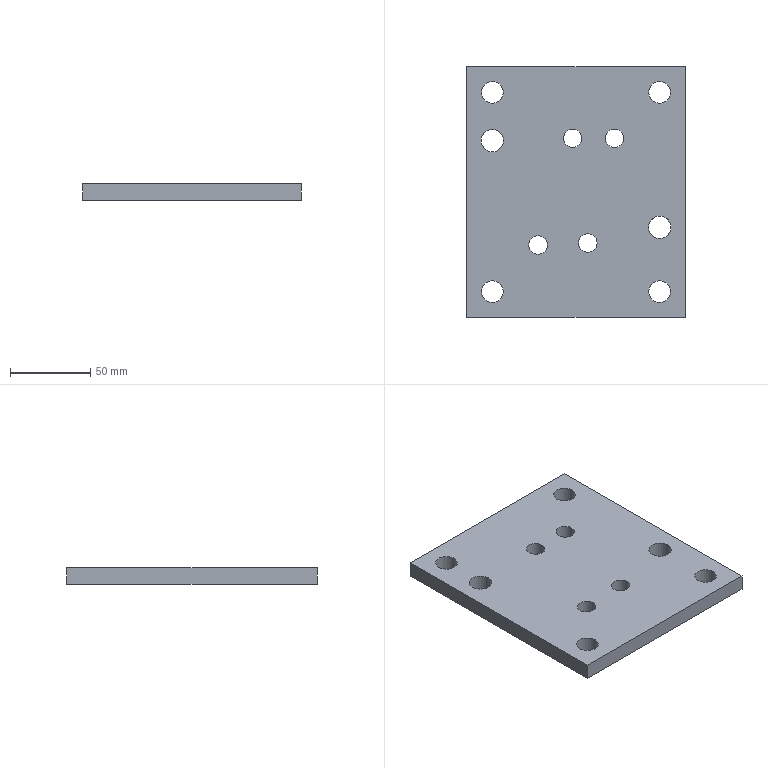Part | NX | features 6 2 | 1 solid | 16 faces | box 136 x 156 x 10 mm | volume 199200 mm3 | cylinder 10 | plane 6 | commonest cylinder face diameters 11.5 x4 13.5 x4 14.001 x2
STEP:
#1=CARTESIAN_POINT('',(3796.562,457.449,91.));
#2=VERTEX_POINT('',#1);
#3=CARTESIAN_POINT('',(3796.562,457.449,101.));
#4=VERTEX_POINT('',#3);
#5=CARTESIAN_POINT('',(3796.562,457.449,91.));
#6=DIRECTION('',(0.,0.,1.));
#7=VECTOR('',#6,1000.);
#8=LINE('',#5,#7);
#9=EDGE_CURVE('',#2,#4,#8,.T.);
#10=ORIENTED_EDGE('',*,*,#9,.F.);
#11=CARTESIAN_POINT('',(3660.562,457.449,91.));
#12=VERTEX_POINT('',#11);
#13=CARTESIAN_POINT('',(3728.562,457.449,91.));
#14=DIRECTION('',(1.,0.,0.));
#15=VECTOR('',#14,1000.);
#16=LINE('',#13,#15);
#17=EDGE_CURVE('',#12,#2,#16,.T.);
#18=ORIENTED_EDGE('',*,*,#17,.F.);
#19=CARTESIAN_POINT('',(3660.562,457.449,101.));
#20=VERTEX_POINT('',#19);
#21=CARTESIAN_POINT('',(3660.562,457.449,91.));
#22=DIRECTION('',(0.,0.,1.));
#23=VECTOR('',#22,1000.);
#24=LINE('',#21,#23);
#25=EDGE_CURVE('',#12,#20,#24,.T.);
#26=ORIENTED_EDGE('',*,*,#25,.T.);
#27=CARTESIAN_POINT('',(3728.562,457.449,101.));
#28=DIRECTION('',(-1.,0.,0.));
#29=VECTOR('',#28,1000.);
#30=LINE('',#27,#29);
#31=EDGE_CURVE('',#4,#20,#30,.T.);
#32=ORIENTED_EDGE('',*,*,#31,.F.);
#33=EDGE_LOOP('',(#10,#18,#26,#32));
#34=FACE_BOUND('',#33,.T.);
#35=CARTESIAN_POINT('',(3728.562,457.449,91.));
#36=DIRECTION('',(0.,1.,0.));
#37=DIRECTION('',(0.,0.,1.));
#38=AXIS2_PLACEMENT_3D('',#35,#36,#37);
#39=PLANE('',#38);
#40=ADVANCED_FACE('',(#34),#39,.T.);
#41=ORIENTED_EDGE('',*,*,#25,.F.);
#42=CARTESIAN_POINT('',(3660.562,301.449,91.));
#43=VERTEX_POINT('',#42);
#44=CARTESIAN_POINT('',(3660.562,379.449,91.));
#45=DIRECTION('',(0.,1.,0.));
#46=VECTOR('',#45,1000.);
#47=LINE('',#44,#46);
#48=EDGE_CURVE('',#43,#12,#47,.T.);
#49=ORIENTED_EDGE('',*,*,#48,.F.);
#50=CARTESIAN_POINT('',(3660.562,301.449,101.));
#51=VERTEX_POINT('',#50);
#52=CARTESIAN_POINT('',(3660.562,301.449,91.));
#53=DIRECTION('',(0.,0.,1.));
#54=VECTOR('',#53,1000.);
#55=LINE('',#52,#54);
#56=EDGE_CURVE('',#43,#51,#55,.T.);
#57=ORIENTED_EDGE('',*,*,#56,.T.);
#58=CARTESIAN_POINT('',(3660.562,379.449,101.));
#59=DIRECTION('',(0.,-1.,0.));
#60=VECTOR('',#59,1000.);
#61=LINE('',#58,#60);
#62=EDGE_CURVE('',#20,#51,#61,.T.);
#63=ORIENTED_EDGE('',*,*,#62,.F.);
#64=EDGE_LOOP('',(#41,#49,#57,#63));
#65=FACE_BOUND('',#64,.T.);
#66=CARTESIAN_POINT('',(3660.562,379.449,91.));
#67=DIRECTION('',(-1.,0.,0.));
#68=DIRECTION('',(0.,0.,-1.));
#69=AXIS2_PLACEMENT_3D('',#66,#67,#68);
#70=PLANE('',#69);
#71=ADVANCED_FACE('',(#65),#70,.T.);
#72=ORIENTED_EDGE('',*,*,#56,.F.);
#73=CARTESIAN_POINT('',(3796.562,301.449,91.));
#74=VERTEX_POINT('',#73);
#75=CARTESIAN_POINT('',(3728.562,301.449,91.));
#76=DIRECTION('',(-1.,0.,0.));
#77=VECTOR('',#76,1000.);
#78=LINE('',#75,#77);
#79=EDGE_CURVE('',#74,#43,#78,.T.);
#80=ORIENTED_EDGE('',*,*,#79,.F.);
#81=CARTESIAN_POINT('',(3796.562,301.449,101.));
#82=VERTEX_POINT('',#81);
#83=CARTESIAN_POINT('',(3796.562,301.449,91.));
#84=DIRECTION('',(0.,0.,1.));
#85=VECTOR('',#84,1000.);
#86=LINE('',#83,#85);
#87=EDGE_CURVE('',#74,#82,#86,.T.);
#88=ORIENTED_EDGE('',*,*,#87,.T.);
#89=CARTESIAN_POINT('',(3728.562,301.449,101.));
#90=DIRECTION('',(1.,0.,0.));
#91=VECTOR('',#90,1000.);
#92=LINE('',#89,#91);
#93=EDGE_CURVE('',#51,#82,#92,.T.);
#94=ORIENTED_EDGE('',*,*,#93,.F.);
#95=EDGE_LOOP('',(#72,#80,#88,#94));
#96=FACE_BOUND('',#95,.T.);
#97=CARTESIAN_POINT('',(3728.562,301.449,91.));
#98=DIRECTION('',(0.,-1.,0.));
#99=DIRECTION('',(0.,0.,-1.));
#100=AXIS2_PLACEMENT_3D('',#97,#98,#99);
#101=PLANE('',#100);
#102=ADVANCED_FACE('',(#96),#101,.T.);
#103=ORIENTED_EDGE('',*,*,#87,.F.);
#104=CARTESIAN_POINT('',(3796.562,379.449,91.));
#105=DIRECTION('',(0.,-1.,0.));
#106=VECTOR('',#105,1000.);
#107=LINE('',#104,#106);
#108=EDGE_CURVE('',#2,#74,#107,.T.);
#109=ORIENTED_EDGE('',*,*,#108,.F.);
#110=ORIENTED_EDGE('',*,*,#9,.T.);
#111=CARTESIAN_POINT('',(3796.562,379.449,101.));
#112=DIRECTION('',(0.,1.,0.));
#113=VECTOR('',#112,1000.);
#114=LINE('',#111,#113);
#115=EDGE_CURVE('',#82,#4,#114,.T.);
#116=ORIENTED_EDGE('',*,*,#115,.F.);
#117=EDGE_LOOP('',(#103,#109,#110,#116));
#118=FACE_BOUND('',#117,.T.);
#119=CARTESIAN_POINT('',(3796.562,379.449,91.));
#120=DIRECTION('',(1.,0.,0.));
#121=DIRECTION('',(0.,0.,1.));
#122=AXIS2_PLACEMENT_3D('',#119,#120,#121);
#123=PLANE('',#122);
#124=ADVANCED_FACE('',(#118),#123,.T.);
#125=CARTESIAN_POINT('',(3683.312,441.449,91.));
#126=VERTEX_POINT('',#125);
#127=CARTESIAN_POINT('',(3676.562,441.449,91.));
#128=DIRECTION('',(0.,0.,-1.));
#129=DIRECTION('',(1.,0.,0.));
#130=AXIS2_PLACEMENT_3D('',#127,#128,#129);
#131=CIRCLE('',#130,6.75);
#132=EDGE_CURVE('',#126,#126,#131,.T.);
#133=ORIENTED_EDGE('',*,*,#132,.T.);
#134=EDGE_LOOP('',(#133));
#135=FACE_BOUND('',#134,.T.);
#136=CARTESIAN_POINT('',(3683.312,441.449,101.));
#137=VERTEX_POINT('',#136);
#138=CARTESIAN_POINT('',(3676.562,441.449,101.));
#139=DIRECTION('',(0.,0.,1.));
#140=DIRECTION('',(1.,0.,0.));
#141=AXIS2_PLACEMENT_3D('',#138,#139,#140);
#142=CIRCLE('',#141,6.75);
#143=EDGE_CURVE('',#137,#137,#142,.T.);
#144=ORIENTED_EDGE('',*,*,#143,.T.);
#145=EDGE_LOOP('',(#144));
#146=FACE_BOUND('',#145,.T.);
#147=CARTESIAN_POINT('',(3676.562,441.449,91.));
#148=DIRECTION('',(0.,0.,1.));
#149=DIRECTION('',(-1.,0.,0.));
#150=AXIS2_PLACEMENT_3D('',#147,#148,#149);
#151=CYLINDRICAL_SURFACE('',#150,6.75);
#152=ADVANCED_FACE('',(#135,#146),#151,.F.);
#153=CARTESIAN_POINT('',(3787.312,317.449,91.));
#154=VERTEX_POINT('',#153);
#155=CARTESIAN_POINT('',(3780.562,317.449,91.));
#156=DIRECTION('',(0.,0.,-1.));
#157=DIRECTION('',(1.,0.,0.));
#158=AXIS2_PLACEMENT_3D('',#155,#156,#157);
#159=CIRCLE('',#158,6.75);
#160=EDGE_CURVE('',#154,#154,#159,.T.);
#161=ORIENTED_EDGE('',*,*,#160,.T.);
#162=EDGE_LOOP('',(#161));
#163=FACE_BOUND('',#162,.T.);
#164=CARTESIAN_POINT('',(3787.312,317.449,101.));
#165=VERTEX_POINT('',#164);
#166=CARTESIAN_POINT('',(3780.562,317.449,101.));
#167=DIRECTION('',(0.,0.,1.));
#168=DIRECTION('',(1.,0.,0.));
#169=AXIS2_PLACEMENT_3D('',#166,#167,#168);
#170=CIRCLE('',#169,6.75);
#171=EDGE_CURVE('',#165,#165,#170,.T.);
#172=ORIENTED_EDGE('',*,*,#171,.T.);
#173=EDGE_LOOP('',(#172));
#174=FACE_BOUND('',#173,.T.);
#175=CARTESIAN_POINT('',(3780.562,317.449,91.));
#176=DIRECTION('',(0.,0.,1.));
#177=DIRECTION('',(-1.,0.,0.));
#178=AXIS2_PLACEMENT_3D('',#175,#176,#177);
#179=CYLINDRICAL_SURFACE('',#178,6.75);
#180=ADVANCED_FACE('',(#163,#174),#179,.F.);
#181=CARTESIAN_POINT('',(3787.312,441.449,91.));
#182=VERTEX_POINT('',#181);
#183=CARTESIAN_POINT('',(3780.562,441.449,91.));
#184=DIRECTION('',(0.,0.,-1.));
#185=DIRECTION('',(1.,0.,0.));
#186=AXIS2_PLACEMENT_3D('',#183,#184,#185);
#187=CIRCLE('',#186,6.75);
#188=EDGE_CURVE('',#182,#182,#187,.T.);
#189=ORIENTED_EDGE('',*,*,#188,.T.);
#190=EDGE_LOOP('',(#189));
#191=FACE_BOUND('',#190,.T.);
#192=CARTESIAN_POINT('',(3787.312,441.449,101.));
#193=VERTEX_POINT('',#192);
#194=CARTESIAN_POINT('',(3780.562,441.449,101.));
#195=DIRECTION('',(0.,0.,1.));
#196=DIRECTION('',(1.,0.,0.));
#197=AXIS2_PLACEMENT_3D('',#194,#195,#196);
#198=CIRCLE('',#197,6.75);
#199=EDGE_CURVE('',#193,#193,#198,.T.);
#200=ORIENTED_EDGE('',*,*,#199,.T.);
#201=EDGE_LOOP('',(#200));
#202=FACE_BOUND('',#201,.T.);
#203=CARTESIAN_POINT('',(3780.562,441.449,91.));
#204=DIRECTION('',(0.,0.,1.));
#205=DIRECTION('',(-1.,0.,0.));
#206=AXIS2_PLACEMENT_3D('',#203,#204,#205);
#207=CYLINDRICAL_SURFACE('',#206,6.75);
#208=ADVANCED_FACE('',(#191,#202),#207,.F.);
#209=CARTESIAN_POINT('',(3683.312,317.449,91.));
#210=VERTEX_POINT('',#209);
#211=CARTESIAN_POINT('',(3676.562,317.449,91.));
#212=DIRECTION('',(0.,0.,-1.));
#213=DIRECTION('',(1.,0.,0.));
#214=AXIS2_PLACEMENT_3D('',#211,#212,#213);
#215=CIRCLE('',#214,6.75);
#216=EDGE_CURVE('',#210,#210,#215,.T.);
#217=ORIENTED_EDGE('',*,*,#216,.T.);
#218=EDGE_LOOP('',(#217));
#219=FACE_BOUND('',#218,.T.);
#220=CARTESIAN_POINT('',(3683.312,317.449,101.));
#221=VERTEX_POINT('',#220);
#222=CARTESIAN_POINT('',(3676.562,317.449,101.));
#223=DIRECTION('',(0.,0.,1.));
#224=DIRECTION('',(1.,0.,0.));
#225=AXIS2_PLACEMENT_3D('',#222,#223,#224);
#226=CIRCLE('',#225,6.75);
#227=EDGE_CURVE('',#221,#221,#226,.T.);
#228=ORIENTED_EDGE('',*,*,#227,.T.);
#229=EDGE_LOOP('',(#228));
#230=FACE_BOUND('',#229,.T.);
#231=CARTESIAN_POINT('',(3676.562,317.449,91.));
#232=DIRECTION('',(0.,0.,1.));
#233=DIRECTION('',(-1.,0.,0.));
#234=AXIS2_PLACEMENT_3D('',#231,#232,#233);
#235=CYLINDRICAL_SURFACE('',#234,6.75);
#236=ADVANCED_FACE('',(#219,#230),#235,.F.);
#237=CARTESIAN_POINT('',(3683.562,411.449,91.));
#238=VERTEX_POINT('',#237);
#239=CARTESIAN_POINT('',(3676.562,411.449,91.));
#240=DIRECTION('',(0.,0.,-1.));
#241=DIRECTION('',(1.,0.,0.));
#242=AXIS2_PLACEMENT_3D('',#239,#240,#241);
#243=CIRCLE('',#242,7.);
#244=EDGE_CURVE('',#238,#238,#243,.T.);
#245=ORIENTED_EDGE('',*,*,#244,.T.);
#246=EDGE_LOOP('',(#245));
#247=FACE_BOUND('',#246,.T.);
#248=CARTESIAN_POINT('',(3683.562,411.449,101.));
#249=VERTEX_POINT('',#248);
#250=CARTESIAN_POINT('',(3676.562,411.449,101.));
#251=DIRECTION('',(0.,0.,1.));
#252=DIRECTION('',(1.,0.,0.));
#253=AXIS2_PLACEMENT_3D('',#250,#251,#252);
#254=CIRCLE('',#253,7.);
#255=EDGE_CURVE('',#249,#249,#254,.T.);
#256=ORIENTED_EDGE('',*,*,#255,.T.);
#257=EDGE_LOOP('',(#256));
#258=FACE_BOUND('',#257,.T.);
#259=CARTESIAN_POINT('',(3676.562,411.449,91.));
#260=DIRECTION('',(0.,0.,1.));
#261=DIRECTION('',(-1.,0.,0.));
#262=AXIS2_PLACEMENT_3D('',#259,#260,#261);
#263=CYLINDRICAL_SURFACE('',#262,7.);
#264=ADVANCED_FACE('',(#247,#258),#263,.F.);
#265=CARTESIAN_POINT('',(3787.562,357.449,91.));
#266=VERTEX_POINT('',#265);
#267=CARTESIAN_POINT('',(3780.562,357.449,91.));
#268=DIRECTION('',(0.,0.,-1.));
#269=DIRECTION('',(1.,0.,0.));
#270=AXIS2_PLACEMENT_3D('',#267,#268,#269);
#271=CIRCLE('',#270,7.);
#272=EDGE_CURVE('',#266,#266,#271,.T.);
#273=ORIENTED_EDGE('',*,*,#272,.T.);
#274=EDGE_LOOP('',(#273));
#275=FACE_BOUND('',#274,.T.);
#276=CARTESIAN_POINT('',(3787.562,357.449,101.));
#277=VERTEX_POINT('',#276);
#278=CARTESIAN_POINT('',(3780.562,357.449,101.));
#279=DIRECTION('',(0.,0.,1.));
#280=DIRECTION('',(1.,0.,0.));
#281=AXIS2_PLACEMENT_3D('',#278,#279,#280);
#282=CIRCLE('',#281,7.);
#283=EDGE_CURVE('',#277,#277,#282,.T.);
#284=ORIENTED_EDGE('',*,*,#283,.T.);
#285=EDGE_LOOP('',(#284));
#286=FACE_BOUND('',#285,.T.);
#287=CARTESIAN_POINT('',(3780.562,357.449,91.));
#288=DIRECTION('',(0.,0.,1.));
#289=DIRECTION('',(-1.,0.,0.));
#290=AXIS2_PLACEMENT_3D('',#287,#288,#289);
#291=CYLINDRICAL_SURFACE('',#290,7.);
#292=ADVANCED_FACE('',(#275,#286),#291,.F.);
#293=CARTESIAN_POINT('',(3699.229,346.424,91.));
#294=VERTEX_POINT('',#293);
#295=CARTESIAN_POINT('',(3704.979,346.424,91.));
#296=DIRECTION('',(0.,0.,1.));
#297=DIRECTION('',(-1.,0.,0.));
#298=AXIS2_PLACEMENT_3D('',#295,#296,#297);
#299=CIRCLE('',#298,5.75);
#300=EDGE_CURVE('',#294,#294,#299,.T.);
#301=ORIENTED_EDGE('',*,*,#300,.T.);
#302=EDGE_LOOP('',(#301));
#303=FACE_BOUND('',#302,.T.);
#304=CARTESIAN_POINT('',(3720.749,412.84,91.));
#305=VERTEX_POINT('',#304);
#306=CARTESIAN_POINT('',(3726.499,412.84,91.));
#307=DIRECTION('',(0.,0.,-1.));
#308=DIRECTION('',(-1.,0.,0.));
#309=AXIS2_PLACEMENT_3D('',#306,#307,#308);
#310=CIRCLE('',#309,5.75);
#311=EDGE_CURVE('',#305,#305,#310,.T.);
#312=ORIENTED_EDGE('',*,*,#311,.F.);
#313=EDGE_LOOP('',(#312));
#314=FACE_BOUND('',#313,.T.);
#315=CARTESIAN_POINT('',(3730.202,347.721,91.));
#316=VERTEX_POINT('',#315);
#317=CARTESIAN_POINT('',(3735.952,347.721,91.));
#318=DIRECTION('',(0.,0.,1.));
#319=DIRECTION('',(-1.,0.,0.));
#320=AXIS2_PLACEMENT_3D('',#317,#318,#319);
#321=CIRCLE('',#320,5.75);
#322=EDGE_CURVE('',#316,#316,#321,.T.);
#323=ORIENTED_EDGE('',*,*,#322,.T.);
#324=EDGE_LOOP('',(#323));
#325=FACE_BOUND('',#324,.T.);
#326=CARTESIAN_POINT('',(3746.749,412.84,91.));
#327=VERTEX_POINT('',#326);
#328=CARTESIAN_POINT('',(3752.499,412.84,91.));
#329=DIRECTION('',(0.,0.,1.));
#330=DIRECTION('',(-1.,0.,0.));
#331=AXIS2_PLACEMENT_3D('',#328,#329,#330);
#332=CIRCLE('',#331,5.75);
#333=EDGE_CURVE('',#327,#327,#332,.T.);
#334=ORIENTED_EDGE('',*,*,#333,.T.);
#335=EDGE_LOOP('',(#334));
#336=FACE_BOUND('',#335,.T.);
#337=ORIENTED_EDGE('',*,*,#244,.F.);
#338=EDGE_LOOP('',(#337));
#339=FACE_BOUND('',#338,.T.);
#340=ORIENTED_EDGE('',*,*,#188,.F.);
#341=EDGE_LOOP('',(#340));
#342=FACE_BOUND('',#341,.T.);
#343=ORIENTED_EDGE('',*,*,#132,.F.);
#344=EDGE_LOOP('',(#343));
#345=FACE_BOUND('',#344,.T.);
#346=ORIENTED_EDGE('',*,*,#108,.T.);
#347=ORIENTED_EDGE('',*,*,#79,.T.);
#348=ORIENTED_EDGE('',*,*,#48,.T.);
#349=ORIENTED_EDGE('',*,*,#17,.T.);
#350=EDGE_LOOP('',(#346,#347,#348,#349));
#351=FACE_BOUND('',#350,.T.);
#352=ORIENTED_EDGE('',*,*,#160,.F.);
#353=EDGE_LOOP('',(#352));
#354=FACE_BOUND('',#353,.T.);
#355=ORIENTED_EDGE('',*,*,#216,.F.);
#356=EDGE_LOOP('',(#355));
#357=FACE_BOUND('',#356,.T.);
#358=ORIENTED_EDGE('',*,*,#272,.F.);
#359=EDGE_LOOP('',(#358));
#360=FACE_BOUND('',#359,.T.);
#361=CARTESIAN_POINT('',(3728.562,379.449,91.));
#362=DIRECTION('',(0.,0.,-1.));
#363=DIRECTION('',(1.,0.,0.));
#364=AXIS2_PLACEMENT_3D('',#361,#362,#363);
#365=PLANE('',#364);
#366=ADVANCED_FACE('',(#303,#314,#325,#336,#339,#342,#345,#351,#354,#357,#360),#365,.T.);
#367=CARTESIAN_POINT('',(3710.729,346.424,101.));
#368=VERTEX_POINT('',#367);
#369=CARTESIAN_POINT('',(3704.979,346.424,101.));
#370=DIRECTION('',(0.,0.,-1.));
#371=DIRECTION('',(1.,0.,0.));
#372=AXIS2_PLACEMENT_3D('',#369,#370,#371);
#373=CIRCLE('',#372,5.75);
#374=EDGE_CURVE('',#368,#368,#373,.T.);
#375=ORIENTED_EDGE('',*,*,#374,.T.);
#376=EDGE_LOOP('',(#375));
#377=FACE_BOUND('',#376,.T.);
#378=CARTESIAN_POINT('',(3732.249,412.84,101.));
#379=VERTEX_POINT('',#378);
#380=CARTESIAN_POINT('',(3726.499,412.84,101.));
#381=DIRECTION('',(0.,0.,1.));
#382=DIRECTION('',(1.,0.,0.));
#383=AXIS2_PLACEMENT_3D('',#380,#381,#382);
#384=CIRCLE('',#383,5.75);
#385=EDGE_CURVE('',#379,#379,#384,.T.);
#386=ORIENTED_EDGE('',*,*,#385,.F.);
#387=EDGE_LOOP('',(#386));
#388=FACE_BOUND('',#387,.T.);
#389=CARTESIAN_POINT('',(3741.702,347.721,101.));
#390=VERTEX_POINT('',#389);
#391=CARTESIAN_POINT('',(3735.952,347.721,101.));
#392=DIRECTION('',(0.,0.,-1.));
#393=DIRECTION('',(1.,0.,0.));
#394=AXIS2_PLACEMENT_3D('',#391,#392,#393);
#395=CIRCLE('',#394,5.75);
#396=EDGE_CURVE('',#390,#390,#395,.T.);
#397=ORIENTED_EDGE('',*,*,#396,.T.);
#398=EDGE_LOOP('',(#397));
#399=FACE_BOUND('',#398,.T.);
#400=CARTESIAN_POINT('',(3758.249,412.84,101.));
#401=VERTEX_POINT('',#400);
#402=CARTESIAN_POINT('',(3752.499,412.84,101.));
#403=DIRECTION('',(0.,0.,-1.));
#404=DIRECTION('',(1.,0.,0.));
#405=AXIS2_PLACEMENT_3D('',#402,#403,#404);
#406=CIRCLE('',#405,5.75);
#407=EDGE_CURVE('',#401,#401,#406,.T.);
#408=ORIENTED_EDGE('',*,*,#407,.T.);
#409=EDGE_LOOP('',(#408));
#410=FACE_BOUND('',#409,.T.);
#411=ORIENTED_EDGE('',*,*,#31,.T.);
#412=ORIENTED_EDGE('',*,*,#62,.T.);
#413=ORIENTED_EDGE('',*,*,#93,.T.);
#414=ORIENTED_EDGE('',*,*,#115,.T.);
#415=EDGE_LOOP('',(#411,#412,#413,#414));
#416=FACE_BOUND('',#415,.T.);
#417=ORIENTED_EDGE('',*,*,#171,.F.);
#418=EDGE_LOOP('',(#417));
#419=FACE_BOUND('',#418,.T.);
#420=ORIENTED_EDGE('',*,*,#227,.F.);
#421=EDGE_LOOP('',(#420));
#422=FACE_BOUND('',#421,.T.);
#423=ORIENTED_EDGE('',*,*,#283,.F.);
#424=EDGE_LOOP('',(#423));
#425=FACE_BOUND('',#424,.T.);
#426=ORIENTED_EDGE('',*,*,#255,.F.);
#427=EDGE_LOOP('',(#426));
#428=FACE_BOUND('',#427,.T.);
#429=ORIENTED_EDGE('',*,*,#199,.F.);
#430=EDGE_LOOP('',(#429));
#431=FACE_BOUND('',#430,.T.);
#432=ORIENTED_EDGE('',*,*,#143,.F.);
#433=EDGE_LOOP('',(#432));
#434=FACE_BOUND('',#433,.T.);
#435=CARTESIAN_POINT('',(3398.5,0.,101.));
#436=DIRECTION('',(0.,0.,1.));
#437=DIRECTION('',(-1.,0.,0.));
#438=AXIS2_PLACEMENT_3D('',#435,#436,#437);
#439=PLANE('',#438);
#440=ADVANCED_FACE('',(#377,#388,#399,#410,#416,#419,#422,#425,#428,#431,#434),#439,.T.);
#441=ORIENTED_EDGE('',*,*,#333,.F.);
#442=EDGE_LOOP('',(#441));
#443=FACE_BOUND('',#442,.T.);
#444=ORIENTED_EDGE('',*,*,#407,.F.);
#445=EDGE_LOOP('',(#444));
#446=FACE_BOUND('',#445,.T.);
#447=CARTESIAN_POINT('',(3752.499,412.84,-91.));
#448=DIRECTION('',(0.,0.,1.));
#449=DIRECTION('',(-1.,0.,0.));
#450=AXIS2_PLACEMENT_3D('',#447,#448,#449);
#451=CYLINDRICAL_SURFACE('',#450,5.75);
#452=ADVANCED_FACE('',(#443,#446),#451,.F.);
#453=ORIENTED_EDGE('',*,*,#322,.F.);
#454=EDGE_LOOP('',(#453));
#455=FACE_BOUND('',#454,.T.);
#456=ORIENTED_EDGE('',*,*,#396,.F.);
#457=EDGE_LOOP('',(#456));
#458=FACE_BOUND('',#457,.T.);
#459=CARTESIAN_POINT('',(3735.952,347.721,-91.));
#460=DIRECTION('',(0.,0.,1.));
#461=DIRECTION('',(-1.,0.,0.));
#462=AXIS2_PLACEMENT_3D('',#459,#460,#461);
#463=CYLINDRICAL_SURFACE('',#462,5.75);
#464=ADVANCED_FACE('',(#455,#458),#463,.F.);
#465=ORIENTED_EDGE('',*,*,#311,.T.);
#466=EDGE_LOOP('',(#465));
#467=FACE_BOUND('',#466,.T.);
#468=ORIENTED_EDGE('',*,*,#385,.T.);
#469=EDGE_LOOP('',(#468));
#470=FACE_BOUND('',#469,.T.);
#471=CARTESIAN_POINT('',(3726.499,412.84,-91.));
#472=DIRECTION('',(0.,0.,1.));
#473=DIRECTION('',(-1.,0.,0.));
#474=AXIS2_PLACEMENT_3D('',#471,#472,#473);
#475=CYLINDRICAL_SURFACE('',#474,5.75);
#476=ADVANCED_FACE('',(#467,#470),#475,.F.);
#477=ORIENTED_EDGE('',*,*,#300,.F.);
#478=EDGE_LOOP('',(#477));
#479=FACE_BOUND('',#478,.T.);
#480=ORIENTED_EDGE('',*,*,#374,.F.);
#481=EDGE_LOOP('',(#480));
#482=FACE_BOUND('',#481,.T.);
#483=CARTESIAN_POINT('',(3704.979,346.424,-91.));
#484=DIRECTION('',(0.,0.,1.));
#485=DIRECTION('',(-1.,0.,0.));
#486=AXIS2_PLACEMENT_3D('',#483,#484,#485);
#487=CYLINDRICAL_SURFACE('',#486,5.75);
#488=ADVANCED_FACE('',(#479,#482),#487,.F.);
#489=CLOSED_SHELL('',(#40,#71,#102,#124,#152,#180,#208,#236,#264,#292,#366,#440,#452,#464,#476,#488));
#490=MANIFOLD_SOLID_BREP('',#489);
#491=(LENGTH_UNIT()NAMED_UNIT(*)SI_UNIT(.MILLI.,.METRE.));
#492=UNCERTAINTY_MEASURE_WITH_UNIT(LENGTH_MEASURE(0.00001),#491,'','');
#493=(NAMED_UNIT(*)PLANE_ANGLE_UNIT()SI_UNIT($,.RADIAN.));
#494=(NAMED_UNIT(*)SI_UNIT($,.STERADIAN.)SOLID_ANGLE_UNIT());
#495=(GEOMETRIC_REPRESENTATION_CONTEXT(3)GLOBAL_UNCERTAINTY_ASSIGNED_CONTEXT((#492))GLOBAL_UNIT_ASSIGNED_CONTEXT((#491,#493,#494))REPRESENTATION_CONTEXT('',''));
#496=ADVANCED_BREP_SHAPE_REPRESENTATION('',(#490),#495);